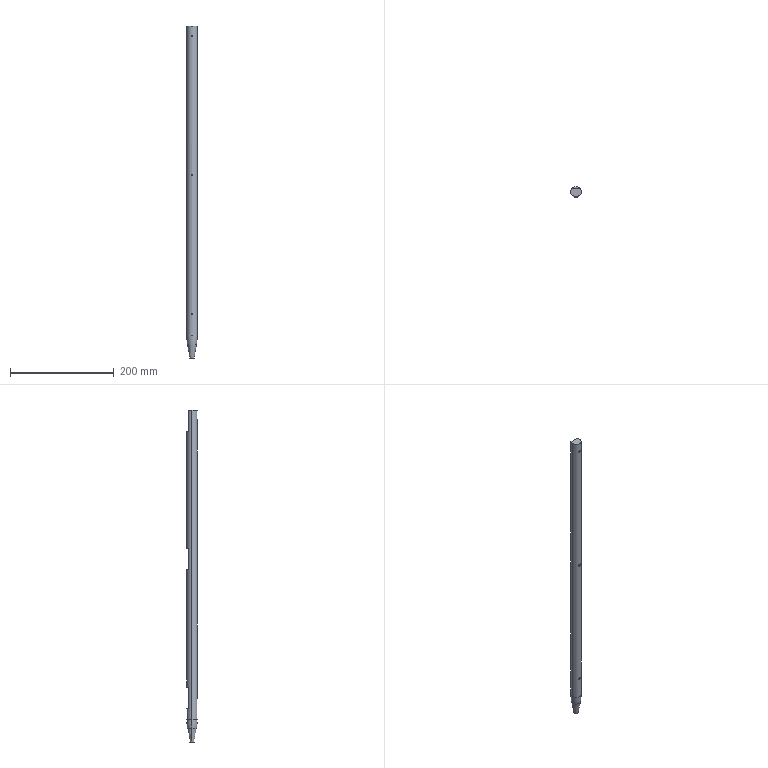Part | STEP file | X77-09002 | 1 solid | 28 faces | box 20 x 20 x 640 mm | volume 189382 mm3 | plane 10 | cylinder 8 | cone 8 | torus 2 | commonest cylinder face diameters 5 x6 20 x2
STEP:
#1=CARTESIAN_POINT('',(-186.5,-272.175,617.5));
#2=VERTEX_POINT('',#1);
#3=CARTESIAN_POINT('',(-186.5,-272.175,622.5));
#4=VERTEX_POINT('',#3);
#5=CARTESIAN_POINT('',(-186.5,-272.175,620.));
#6=DIRECTION('',(0.,1.,0.));
#7=DIRECTION('',(0.,0.,1.));
#8=AXIS2_PLACEMENT_3D('',#5,#6,#7);
#9=CIRCLE('',#8,2.5);
#10=EDGE_CURVE('',#2,#4,#9,.T.);
#11=ORIENTED_EDGE('',*,*,#10,.F.);
#12=CARTESIAN_POINT('',(-186.5,-257.175,617.5));
#13=VERTEX_POINT('',#12);
#14=CARTESIAN_POINT('',(-186.5,-257.175,617.5));
#15=DIRECTION('',(0.,1.,0.));
#16=VECTOR('',#15,1000.);
#17=LINE('',#14,#16);
#18=EDGE_CURVE('',#2,#13,#17,.T.);
#19=ORIENTED_EDGE('',*,*,#18,.T.);
#20=CARTESIAN_POINT('',(-186.5,-257.175,622.5));
#21=VERTEX_POINT('',#20);
#22=CARTESIAN_POINT('',(-186.5,-257.175,620.));
#23=DIRECTION('',(0.,1.,0.));
#24=DIRECTION('',(0.,0.,1.));
#25=AXIS2_PLACEMENT_3D('',#22,#23,#24);
#26=CIRCLE('',#25,2.5);
#27=EDGE_CURVE('',#13,#21,#26,.T.);
#28=ORIENTED_EDGE('',*,*,#27,.T.);
#29=CARTESIAN_POINT('',(-186.5,-257.175,622.5));
#30=DIRECTION('',(0.,1.,0.));
#31=VECTOR('',#30,1000.);
#32=LINE('',#29,#31);
#33=EDGE_CURVE('',#4,#21,#32,.T.);
#34=ORIENTED_EDGE('',*,*,#33,.F.);
#35=EDGE_LOOP('',(#11,#19,#28,#34));
#36=FACE_OUTER_BOUND('',#35,.T.);
#37=CARTESIAN_POINT('',(-186.5,-257.175,620.));
#38=DIRECTION('',(0.,1.,0.));
#39=DIRECTION('',(0.,0.,1.));
#40=AXIS2_PLACEMENT_3D('',#37,#38,#39);
#41=CYLINDRICAL_SURFACE('',#40,2.5);
#42=ADVANCED_FACE('',(#36),#41,.F.);
#43=CARTESIAN_POINT('',(-186.5,-273.175,619.164));
#44=VERTEX_POINT('',#43);
#45=CARTESIAN_POINT('',(-186.5,-273.175,620.836));
#46=VERTEX_POINT('',#45);
#47=CARTESIAN_POINT('',(-186.5,-273.175,619.164));
#48=CARTESIAN_POINT('',(-186.613,-273.175,619.164));
#49=CARTESIAN_POINT('',(-186.728,-273.173,619.184));
#50=CARTESIAN_POINT('',(-186.943,-273.166,619.264));
#51=CARTESIAN_POINT('',(-187.041,-273.161,619.322));
#52=CARTESIAN_POINT('',(-187.212,-273.15,619.475));
#53=CARTESIAN_POINT('',(-187.281,-273.145,619.566));
#54=CARTESIAN_POINT('',(-187.378,-273.137,619.773));
#55=CARTESIAN_POINT('',(-187.404,-273.134,619.886));
#56=CARTESIAN_POINT('',(-187.404,-273.134,620.113));
#57=CARTESIAN_POINT('',(-187.378,-273.137,620.227));
#58=CARTESIAN_POINT('',(-187.282,-273.145,620.433));
#59=CARTESIAN_POINT('',(-187.212,-273.15,620.526));
#60=CARTESIAN_POINT('',(-186.955,-273.166,620.754));
#61=CARTESIAN_POINT('',(-186.728,-273.175,620.836));
#62=CARTESIAN_POINT('',(-186.5,-273.175,620.836));
#63=B_SPLINE_CURVE_WITH_KNOTS('',3,(#47,#48,#49,#50,#51,#52,#53,#54,#55,#56,#57,#58,#59,#60,#61,#62),.UNSPECIFIED.,.F.,.F.,(4,2,2,2,2,2,2,4),(0.00507,0.005409,0.005749,0.006088,0.006428,0.006768,0.007107,0.007786),.UNSPECIFIED.);
#64=EDGE_CURVE('',#44,#46,#63,.T.);
#65=ORIENTED_EDGE('',*,*,#64,.F.);
#66=CARTESIAN_POINT('',(-186.5,-272.175,617.5));
#67=DIRECTION('',(0.,0.515,-0.8572));
#68=VECTOR('',#67,1000.);
#69=LINE('',#66,#68);
#70=EDGE_CURVE('',#44,#2,#69,.T.);
#71=ORIENTED_EDGE('',*,*,#70,.T.);
#72=ORIENTED_EDGE('',*,*,#10,.T.);
#73=CARTESIAN_POINT('',(-186.5,-272.175,622.5));
#74=DIRECTION('',(0.,0.515,0.8572));
#75=VECTOR('',#74,1000.);
#76=LINE('',#73,#75);
#77=EDGE_CURVE('',#46,#4,#76,.T.);
#78=ORIENTED_EDGE('',*,*,#77,.F.);
#79=EDGE_LOOP('',(#65,#71,#72,#78));
#80=FACE_OUTER_BOUND('',#79,.T.);
#81=CARTESIAN_POINT('',(-186.5,-272.175,620.));
#82=DIRECTION('',(0.,1.,0.));
#83=DIRECTION('',(0.,0.,1.));
#84=AXIS2_PLACEMENT_3D('',#81,#82,#83);
#85=CONICAL_SURFACE('',#84,2.5,1.03);
#86=ADVANCED_FACE('',(#80),#85,.F.);
#87=CARTESIAN_POINT('',(-186.5,-272.175,350.));
#88=VERTEX_POINT('',#87);
#89=CARTESIAN_POINT('',(-186.5,-272.175,355.));
#90=VERTEX_POINT('',#89);
#91=CARTESIAN_POINT('',(-186.5,-272.175,352.5));
#92=DIRECTION('',(0.,1.,0.));
#93=DIRECTION('',(0.,0.,1.));
#94=AXIS2_PLACEMENT_3D('',#91,#92,#93);
#95=CIRCLE('',#94,2.5);
#96=EDGE_CURVE('',#88,#90,#95,.T.);
#97=ORIENTED_EDGE('',*,*,#96,.F.);
#98=CARTESIAN_POINT('',(-186.5,-257.175,350.));
#99=VERTEX_POINT('',#98);
#100=CARTESIAN_POINT('',(-186.5,-257.175,350.));
#101=DIRECTION('',(0.,1.,0.));
#102=VECTOR('',#101,1000.);
#103=LINE('',#100,#102);
#104=EDGE_CURVE('',#88,#99,#103,.T.);
#105=ORIENTED_EDGE('',*,*,#104,.T.);
#106=CARTESIAN_POINT('',(-186.5,-257.175,355.));
#107=VERTEX_POINT('',#106);
#108=CARTESIAN_POINT('',(-186.5,-257.175,352.5));
#109=DIRECTION('',(0.,-1.,0.));
#110=DIRECTION('',(0.,0.,1.));
#111=AXIS2_PLACEMENT_3D('',#108,#109,#110);
#112=CIRCLE('',#111,2.5);
#113=EDGE_CURVE('',#107,#99,#112,.T.);
#114=ORIENTED_EDGE('',*,*,#113,.F.);
#115=CARTESIAN_POINT('',(-186.5,-257.175,355.));
#116=DIRECTION('',(0.,1.,0.));
#117=VECTOR('',#116,1000.);
#118=LINE('',#115,#117);
#119=EDGE_CURVE('',#90,#107,#118,.T.);
#120=ORIENTED_EDGE('',*,*,#119,.F.);
#121=EDGE_LOOP('',(#97,#105,#114,#120));
#122=FACE_OUTER_BOUND('',#121,.T.);
#123=CARTESIAN_POINT('',(-186.5,-257.175,352.5));
#124=DIRECTION('',(0.,1.,0.));
#125=DIRECTION('',(0.,0.,1.));
#126=AXIS2_PLACEMENT_3D('',#123,#124,#125);
#127=CYLINDRICAL_SURFACE('',#126,2.5);
#128=ADVANCED_FACE('',(#122),#127,.F.);
#129=CARTESIAN_POINT('',(-186.5,-273.175,351.664));
#130=VERTEX_POINT('',#129);
#131=CARTESIAN_POINT('',(-186.5,-273.175,353.336));
#132=VERTEX_POINT('',#131);
#133=CARTESIAN_POINT('',(-186.5,-273.175,351.664));
#134=CARTESIAN_POINT('',(-186.729,-273.175,351.664));
#135=CARTESIAN_POINT('',(-186.954,-273.166,351.745));
#136=CARTESIAN_POINT('',(-187.211,-273.15,351.974));
#137=CARTESIAN_POINT('',(-187.281,-273.145,352.065));
#138=CARTESIAN_POINT('',(-187.378,-273.137,352.272));
#139=CARTESIAN_POINT('',(-187.404,-273.134,352.386));
#140=CARTESIAN_POINT('',(-187.404,-273.134,352.614));
#141=CARTESIAN_POINT('',(-187.378,-273.137,352.727));
#142=CARTESIAN_POINT('',(-187.281,-273.145,352.935));
#143=CARTESIAN_POINT('',(-187.21,-273.15,353.027));
#144=CARTESIAN_POINT('',(-186.956,-273.166,353.253));
#145=CARTESIAN_POINT('',(-186.727,-273.175,353.336));
#146=CARTESIAN_POINT('',(-186.5,-273.175,353.336));
#147=B_SPLINE_CURVE_WITH_KNOTS('',3,(#133,#134,#135,#136,#137,#138,#139,#140,#141,#142,#143,#144,#145,#146),.UNSPECIFIED.,.F.,.F.,(4,2,2,2,2,2,4),(0.004257,0.004938,0.005279,0.005619,0.00596,0.006301,0.006982),.UNSPECIFIED.);
#148=EDGE_CURVE('',#130,#132,#147,.T.);
#149=ORIENTED_EDGE('',*,*,#148,.F.);
#150=CARTESIAN_POINT('',(-186.5,-272.175,350.));
#151=DIRECTION('',(0.,0.515,-0.8572));
#152=VECTOR('',#151,1000.);
#153=LINE('',#150,#152);
#154=EDGE_CURVE('',#130,#88,#153,.T.);
#155=ORIENTED_EDGE('',*,*,#154,.T.);
#156=ORIENTED_EDGE('',*,*,#96,.T.);
#157=CARTESIAN_POINT('',(-186.5,-272.175,355.));
#158=DIRECTION('',(0.,0.515,0.8572));
#159=VECTOR('',#158,1000.);
#160=LINE('',#157,#159);
#161=EDGE_CURVE('',#132,#90,#160,.T.);
#162=ORIENTED_EDGE('',*,*,#161,.F.);
#163=EDGE_LOOP('',(#149,#155,#156,#162));
#164=FACE_OUTER_BOUND('',#163,.T.);
#165=CARTESIAN_POINT('',(-186.5,-272.175,352.5));
#166=DIRECTION('',(0.,1.,0.));
#167=DIRECTION('',(0.,0.,1.));
#168=AXIS2_PLACEMENT_3D('',#165,#166,#167);
#169=CONICAL_SURFACE('',#168,2.5,1.03);
#170=ADVANCED_FACE('',(#164),#169,.F.);
#171=CARTESIAN_POINT('',(-186.5,-272.175,82.5));
#172=VERTEX_POINT('',#171);
#173=CARTESIAN_POINT('',(-186.5,-272.175,87.5));
#174=VERTEX_POINT('',#173);
#175=CARTESIAN_POINT('',(-186.5,-272.175,85.));
#176=DIRECTION('',(0.,1.,0.));
#177=DIRECTION('',(0.,0.,1.));
#178=AXIS2_PLACEMENT_3D('',#175,#176,#177);
#179=CIRCLE('',#178,2.5);
#180=EDGE_CURVE('',#172,#174,#179,.T.);
#181=ORIENTED_EDGE('',*,*,#180,.F.);
#182=CARTESIAN_POINT('',(-186.5,-257.175,82.5));
#183=VERTEX_POINT('',#182);
#184=CARTESIAN_POINT('',(-186.5,-257.175,82.5));
#185=DIRECTION('',(0.,1.,0.));
#186=VECTOR('',#185,1000.);
#187=LINE('',#184,#186);
#188=EDGE_CURVE('',#172,#183,#187,.T.);
#189=ORIENTED_EDGE('',*,*,#188,.T.);
#190=CARTESIAN_POINT('',(-186.5,-257.175,87.5));
#191=VERTEX_POINT('',#190);
#192=CARTESIAN_POINT('',(-186.5,-257.175,85.));
#193=DIRECTION('',(0.,-1.,0.));
#194=DIRECTION('',(0.,0.,1.));
#195=AXIS2_PLACEMENT_3D('',#192,#193,#194);
#196=CIRCLE('',#195,2.5);
#197=EDGE_CURVE('',#191,#183,#196,.T.);
#198=ORIENTED_EDGE('',*,*,#197,.F.);
#199=CARTESIAN_POINT('',(-186.5,-257.175,87.5));
#200=DIRECTION('',(0.,1.,0.));
#201=VECTOR('',#200,1000.);
#202=LINE('',#199,#201);
#203=EDGE_CURVE('',#174,#191,#202,.T.);
#204=ORIENTED_EDGE('',*,*,#203,.F.);
#205=EDGE_LOOP('',(#181,#189,#198,#204));
#206=FACE_OUTER_BOUND('',#205,.T.);
#207=CARTESIAN_POINT('',(-186.5,-257.175,85.));
#208=DIRECTION('',(0.,1.,0.));
#209=DIRECTION('',(0.,0.,1.));
#210=AXIS2_PLACEMENT_3D('',#207,#208,#209);
#211=CYLINDRICAL_SURFACE('',#210,2.5);
#212=ADVANCED_FACE('',(#206),#211,.F.);
#213=CARTESIAN_POINT('',(-186.5,-273.175,84.164));
#214=VERTEX_POINT('',#213);
#215=CARTESIAN_POINT('',(-186.5,-273.175,85.836));
#216=VERTEX_POINT('',#215);
#217=CARTESIAN_POINT('',(-186.5,-273.175,84.164));
#218=CARTESIAN_POINT('',(-186.729,-273.175,84.164));
#219=CARTESIAN_POINT('',(-186.954,-273.166,84.245));
#220=CARTESIAN_POINT('',(-187.211,-273.15,84.474));
#221=CARTESIAN_POINT('',(-187.281,-273.145,84.565));
#222=CARTESIAN_POINT('',(-187.378,-273.137,84.772));
#223=CARTESIAN_POINT('',(-187.404,-273.134,84.886));
#224=CARTESIAN_POINT('',(-187.404,-273.134,85.114));
#225=CARTESIAN_POINT('',(-187.378,-273.137,85.227));
#226=CARTESIAN_POINT('',(-187.281,-273.145,85.435));
#227=CARTESIAN_POINT('',(-187.21,-273.15,85.527));
#228=CARTESIAN_POINT('',(-186.956,-273.166,85.753));
#229=CARTESIAN_POINT('',(-186.727,-273.175,85.836));
#230=CARTESIAN_POINT('',(-186.5,-273.175,85.836));
#231=B_SPLINE_CURVE_WITH_KNOTS('',3,(#217,#218,#219,#220,#221,#222,#223,#224,#225,#226,#227,#228,#229,#230),.UNSPECIFIED.,.F.,.F.,(4,2,2,2,2,2,4),(0.004257,0.004938,0.005279,0.005619,0.00596,0.006301,0.006982),.UNSPECIFIED.);
#232=EDGE_CURVE('',#214,#216,#231,.T.);
#233=ORIENTED_EDGE('',*,*,#232,.F.);
#234=CARTESIAN_POINT('',(-186.5,-272.175,82.5));
#235=DIRECTION('',(0.,0.515,-0.8572));
#236=VECTOR('',#235,1000.);
#237=LINE('',#234,#236);
#238=EDGE_CURVE('',#214,#172,#237,.T.);
#239=ORIENTED_EDGE('',*,*,#238,.T.);
#240=ORIENTED_EDGE('',*,*,#180,.T.);
#241=CARTESIAN_POINT('',(-186.5,-272.175,87.5));
#242=DIRECTION('',(0.,0.515,0.8572));
#243=VECTOR('',#242,1000.);
#244=LINE('',#241,#243);
#245=EDGE_CURVE('',#216,#174,#244,.T.);
#246=ORIENTED_EDGE('',*,*,#245,.F.);
#247=EDGE_LOOP('',(#233,#239,#240,#246));
#248=FACE_OUTER_BOUND('',#247,.T.);
#249=CARTESIAN_POINT('',(-186.5,-272.175,85.));
#250=DIRECTION('',(0.,1.,0.));
#251=DIRECTION('',(0.,0.,1.));
#252=AXIS2_PLACEMENT_3D('',#249,#250,#251);
#253=CONICAL_SURFACE('',#252,2.5,1.03);
#254=ADVANCED_FACE('',(#248),#253,.F.);
#255=CARTESIAN_POINT('',(-176.5,-263.175,42.777));
#256=VERTEX_POINT('',#255);
#257=CARTESIAN_POINT('',(-196.5,-263.175,42.777));
#258=VERTEX_POINT('',#257);
#259=CARTESIAN_POINT('',(-186.5,-263.175,42.777));
#260=DIRECTION('',(0.,0.,1.));
#261=DIRECTION('',(-1.,0.,0.));
#262=AXIS2_PLACEMENT_3D('',#259,#260,#261);
#263=CIRCLE('',#262,10.);
#264=EDGE_CURVE('',#256,#258,#263,.T.);
#265=ORIENTED_EDGE('',*,*,#264,.F.);
#266=CARTESIAN_POINT('',(-178.019,-263.175,25.412));
#267=VERTEX_POINT('',#266);
#268=CARTESIAN_POINT('',(-276.5,-263.175,42.777));
#269=DIRECTION('',(0.,1.,0.));
#270=DIRECTION('',(-1.,0.,0.));
#271=AXIS2_PLACEMENT_3D('',#268,#269,#270);
#272=CIRCLE('',#271,100.);
#273=EDGE_CURVE('',#256,#267,#272,.T.);
#274=ORIENTED_EDGE('',*,*,#273,.T.);
#275=CARTESIAN_POINT('',(-194.981,-263.175,25.412));
#276=VERTEX_POINT('',#275);
#277=CARTESIAN_POINT('',(-186.5,-263.175,25.412));
#278=DIRECTION('',(0.,0.,-1.));
#279=DIRECTION('',(1.,0.,0.));
#280=AXIS2_PLACEMENT_3D('',#277,#278,#279);
#281=CIRCLE('',#280,8.481);
#282=EDGE_CURVE('',#276,#267,#281,.T.);
#283=ORIENTED_EDGE('',*,*,#282,.F.);
#284=CARTESIAN_POINT('',(-96.5,-263.175,42.777));
#285=DIRECTION('',(0.,-1.,0.));
#286=DIRECTION('',(0.,0.,-1.));
#287=AXIS2_PLACEMENT_3D('',#284,#285,#286);
#288=CIRCLE('',#287,100.);
#289=EDGE_CURVE('',#258,#276,#288,.T.);
#290=ORIENTED_EDGE('',*,*,#289,.F.);
#291=EDGE_LOOP('',(#265,#274,#283,#290));
#292=FACE_OUTER_BOUND('',#291,.T.);
#293=CARTESIAN_POINT('',(-186.5,-263.175,42.777));
#294=DIRECTION('',(0.,0.,-1.));
#295=DIRECTION('',(-1.,0.,0.));
#296=AXIS2_PLACEMENT_3D('',#293,#294,#295);
#297=TOROIDAL_SURFACE('',#296,-90.,100.);
#298=ADVANCED_FACE('',(#292),#297,.T.);
#299=CARTESIAN_POINT('',(-190.5,-263.175,0.));
#300=VERTEX_POINT('',#299);
#301=CARTESIAN_POINT('',(-182.5,-263.175,0.));
#302=VERTEX_POINT('',#301);
#303=CARTESIAN_POINT('',(-186.5,-263.175,0.));
#304=DIRECTION('',(0.,0.,-1.));
#305=DIRECTION('',(1.,0.,0.));
#306=AXIS2_PLACEMENT_3D('',#303,#304,#305);
#307=CIRCLE('',#306,4.);
#308=EDGE_CURVE('',#300,#302,#307,.T.);
#309=ORIENTED_EDGE('',*,*,#308,.F.);
#310=CARTESIAN_POINT('',(-196.5,-263.175,34.028));
#311=DIRECTION('',(-0.1736,0.,0.9848));
#312=VECTOR('',#311,1000.);
#313=LINE('',#310,#312);
#314=EDGE_CURVE('',#300,#276,#313,.T.);
#315=ORIENTED_EDGE('',*,*,#314,.T.);
#316=ORIENTED_EDGE('',*,*,#282,.T.);
#317=CARTESIAN_POINT('',(-176.5,-263.175,34.028));
#318=DIRECTION('',(0.1736,0.,0.9848));
#319=VECTOR('',#318,1000.);
#320=LINE('',#317,#319);
#321=EDGE_CURVE('',#302,#267,#320,.T.);
#322=ORIENTED_EDGE('',*,*,#321,.F.);
#323=EDGE_LOOP('',(#309,#315,#316,#322));
#324=FACE_OUTER_BOUND('',#323,.T.);
#325=CARTESIAN_POINT('',(-186.5,-263.175,34.028));
#326=DIRECTION('',(0.,0.,1.));
#327=DIRECTION('',(1.,0.,0.));
#328=AXIS2_PLACEMENT_3D('',#325,#326,#327);
#329=CONICAL_SURFACE('',#328,10.,0.1745);
#330=ADVANCED_FACE('',(#324),#329,.T.);
#331=CARTESIAN_POINT('',(-178.5,-257.175,106.));
#332=VERTEX_POINT('',#331);
#333=CARTESIAN_POINT('',(-178.5,-257.175,65.));
#334=VERTEX_POINT('',#333);
#335=CARTESIAN_POINT('',(-178.5,-257.175,640.));
#336=DIRECTION('',(0.,0.,-1.));
#337=VECTOR('',#336,1000.);
#338=LINE('',#335,#337);
#339=EDGE_CURVE('',#332,#334,#338,.T.);
#340=ORIENTED_EDGE('',*,*,#339,.F.);
#341=CARTESIAN_POINT('',(-194.5,-257.175,106.));
#342=VERTEX_POINT('',#341);
#343=CARTESIAN_POINT('',(-186.5,-263.175,106.));
#344=DIRECTION('',(0.,0.,-1.));
#345=DIRECTION('',(-1.,0.,0.));
#346=AXIS2_PLACEMENT_3D('',#343,#344,#345);
#347=CIRCLE('',#346,10.);
#348=EDGE_CURVE('',#342,#332,#347,.T.);
#349=ORIENTED_EDGE('',*,*,#348,.F.);
#350=CARTESIAN_POINT('',(-194.5,-257.175,65.));
#351=VERTEX_POINT('',#350);
#352=CARTESIAN_POINT('',(-194.5,-257.175,640.));
#353=DIRECTION('',(0.,0.,1.));
#354=VECTOR('',#353,1000.);
#355=LINE('',#352,#354);
#356=EDGE_CURVE('',#351,#342,#355,.T.);
#357=ORIENTED_EDGE('',*,*,#356,.F.);
#358=CARTESIAN_POINT('',(-186.5,-263.175,65.));
#359=DIRECTION('',(0.,0.,1.));
#360=DIRECTION('',(1.,0.,0.));
#361=AXIS2_PLACEMENT_3D('',#358,#359,#360);
#362=CIRCLE('',#361,10.);
#363=EDGE_CURVE('',#334,#351,#362,.T.);
#364=ORIENTED_EDGE('',*,*,#363,.F.);
#365=EDGE_LOOP('',(#340,#349,#357,#364));
#366=FACE_BOUND('',#365,.T.);
#367=CARTESIAN_POINT('',(-178.5,-257.175,373.));
#368=VERTEX_POINT('',#367);
#369=CARTESIAN_POINT('',(-178.5,-257.175,332.));
#370=VERTEX_POINT('',#369);
#371=CARTESIAN_POINT('',(-178.5,-257.175,640.));
#372=DIRECTION('',(0.,0.,-1.));
#373=VECTOR('',#372,1000.);
#374=LINE('',#371,#373);
#375=EDGE_CURVE('',#368,#370,#374,.T.);
#376=ORIENTED_EDGE('',*,*,#375,.F.);
#377=CARTESIAN_POINT('',(-194.5,-257.175,373.));
#378=VERTEX_POINT('',#377);
#379=CARTESIAN_POINT('',(-186.5,-263.175,373.));
#380=DIRECTION('',(0.,0.,-1.));
#381=DIRECTION('',(-1.,0.,0.));
#382=AXIS2_PLACEMENT_3D('',#379,#380,#381);
#383=CIRCLE('',#382,10.);
#384=EDGE_CURVE('',#378,#368,#383,.T.);
#385=ORIENTED_EDGE('',*,*,#384,.F.);
#386=CARTESIAN_POINT('',(-194.5,-257.175,332.));
#387=VERTEX_POINT('',#386);
#388=CARTESIAN_POINT('',(-194.5,-257.175,640.));
#389=DIRECTION('',(0.,0.,1.));
#390=VECTOR('',#389,1000.);
#391=LINE('',#388,#390);
#392=EDGE_CURVE('',#387,#378,#391,.T.);
#393=ORIENTED_EDGE('',*,*,#392,.F.);
#394=CARTESIAN_POINT('',(-186.5,-263.175,332.));
#395=DIRECTION('',(0.,0.,1.));
#396=DIRECTION('',(1.,0.,0.));
#397=AXIS2_PLACEMENT_3D('',#394,#395,#396);
#398=CIRCLE('',#397,10.);
#399=EDGE_CURVE('',#370,#387,#398,.T.);
#400=ORIENTED_EDGE('',*,*,#399,.F.);
#401=EDGE_LOOP('',(#376,#385,#393,#400));
#402=FACE_BOUND('',#401,.T.);
#403=CARTESIAN_POINT('',(-176.5,-263.175,640.));
#404=VERTEX_POINT('',#403);
#405=CARTESIAN_POINT('',(-178.5,-257.175,640.));
#406=VERTEX_POINT('',#405);
#407=CARTESIAN_POINT('',(-186.5,-263.175,640.));
#408=DIRECTION('',(0.,0.,1.));
#409=DIRECTION('',(1.,0.,0.));
#410=AXIS2_PLACEMENT_3D('',#407,#408,#409);
#411=CIRCLE('',#410,10.);
#412=EDGE_CURVE('',#404,#406,#411,.T.);
#413=ORIENTED_EDGE('',*,*,#412,.F.);
#414=CARTESIAN_POINT('',(-176.5,-263.175,640.));
#415=DIRECTION('',(0.,0.,-1.));
#416=VECTOR('',#415,1000.);
#417=LINE('',#414,#416);
#418=EDGE_CURVE('',#404,#256,#417,.T.);
#419=ORIENTED_EDGE('',*,*,#418,.T.);
#420=ORIENTED_EDGE('',*,*,#264,.T.);
#421=CARTESIAN_POINT('',(-196.5,-263.175,640.));
#422=VERTEX_POINT('',#421);
#423=CARTESIAN_POINT('',(-196.5,-263.175,640.));
#424=DIRECTION('',(0.,0.,-1.));
#425=VECTOR('',#424,1000.);
#426=LINE('',#423,#425);
#427=EDGE_CURVE('',#422,#258,#426,.T.);
#428=ORIENTED_EDGE('',*,*,#427,.F.);
#429=CARTESIAN_POINT('',(-194.5,-257.175,640.));
#430=VERTEX_POINT('',#429);
#431=CARTESIAN_POINT('',(-186.5,-263.175,640.));
#432=DIRECTION('',(0.,0.,1.));
#433=DIRECTION('',(1.,0.,0.));
#434=AXIS2_PLACEMENT_3D('',#431,#432,#433);
#435=CIRCLE('',#434,10.);
#436=EDGE_CURVE('',#430,#422,#435,.T.);
#437=ORIENTED_EDGE('',*,*,#436,.F.);
#438=CARTESIAN_POINT('',(-194.5,-257.175,599.));
#439=VERTEX_POINT('',#438);
#440=CARTESIAN_POINT('',(-194.5,-257.175,640.));
#441=DIRECTION('',(0.,0.,-1.));
#442=VECTOR('',#441,1000.);
#443=LINE('',#440,#442);
#444=EDGE_CURVE('',#430,#439,#443,.T.);
#445=ORIENTED_EDGE('',*,*,#444,.T.);
#446=CARTESIAN_POINT('',(-178.5,-257.175,599.));
#447=VERTEX_POINT('',#446);
#448=CARTESIAN_POINT('',(-186.5,-263.175,599.));
#449=DIRECTION('',(0.,0.,-1.));
#450=DIRECTION('',(-1.,0.,0.));
#451=AXIS2_PLACEMENT_3D('',#448,#449,#450);
#452=CIRCLE('',#451,10.);
#453=EDGE_CURVE('',#439,#447,#452,.T.);
#454=ORIENTED_EDGE('',*,*,#453,.T.);
#455=CARTESIAN_POINT('',(-178.5,-257.175,640.));
#456=DIRECTION('',(0.,0.,1.));
#457=VECTOR('',#456,1000.);
#458=LINE('',#455,#457);
#459=EDGE_CURVE('',#447,#406,#458,.T.);
#460=ORIENTED_EDGE('',*,*,#459,.T.);
#461=EDGE_LOOP('',(#413,#419,#420,#428,#437,#445,#454,#460));
#462=FACE_OUTER_BOUND('',#461,.T.);
#463=CARTESIAN_POINT('',(-186.5,-263.175,640.));
#464=DIRECTION('',(0.,0.,-1.));
#465=DIRECTION('',(-1.,0.,0.));
#466=AXIS2_PLACEMENT_3D('',#463,#464,#465);
#467=CYLINDRICAL_SURFACE('',#466,10.);
#468=ADVANCED_FACE('',(#366,#402,#462),#467,.T.);
#469=ORIENTED_EDGE('',*,*,#418,.F.);
#470=CARTESIAN_POINT('',(-186.5,-263.175,640.));
#471=DIRECTION('',(0.,0.,1.));
#472=DIRECTION('',(1.,0.,0.));
#473=AXIS2_PLACEMENT_3D('',#470,#471,#472);
#474=CIRCLE('',#473,10.);
#475=EDGE_CURVE('',#422,#404,#474,.T.);
#476=ORIENTED_EDGE('',*,*,#475,.F.);
#477=ORIENTED_EDGE('',*,*,#427,.T.);
#478=CARTESIAN_POINT('',(-186.5,-263.175,42.777));
#479=DIRECTION('',(0.,0.,1.));
#480=DIRECTION('',(-1.,0.,0.));
#481=AXIS2_PLACEMENT_3D('',#478,#479,#480);
#482=CIRCLE('',#481,10.);
#483=EDGE_CURVE('',#258,#256,#482,.T.);
#484=ORIENTED_EDGE('',*,*,#483,.T.);
#485=EDGE_LOOP('',(#469,#476,#477,#484));
#486=FACE_OUTER_BOUND('',#485,.T.);
#487=CARTESIAN_POINT('',(-186.5,-273.175,620.836));
#488=CARTESIAN_POINT('',(-186.386,-273.175,620.836));
#489=CARTESIAN_POINT('',(-186.272,-273.173,620.815));
#490=CARTESIAN_POINT('',(-186.059,-273.166,620.737));
#491=CARTESIAN_POINT('',(-185.959,-273.161,620.678));
#492=CARTESIAN_POINT('',(-185.79,-273.15,620.527));
#493=CARTESIAN_POINT('',(-185.719,-273.145,620.434));
#494=CARTESIAN_POINT('',(-185.623,-273.137,620.23));
#495=CARTESIAN_POINT('',(-185.596,-273.134,620.115));
#496=CARTESIAN_POINT('',(-185.596,-273.134,619.888));
#497=CARTESIAN_POINT('',(-185.621,-273.137,619.774));
#498=CARTESIAN_POINT('',(-185.718,-273.145,619.566));
#499=CARTESIAN_POINT('',(-185.789,-273.15,619.474));
#500=CARTESIAN_POINT('',(-186.044,-273.166,619.247));
#501=CARTESIAN_POINT('',(-186.273,-273.175,619.164));
#502=CARTESIAN_POINT('',(-186.5,-273.175,619.164));
#503=B_SPLINE_CURVE_WITH_KNOTS('',3,(#487,#488,#489,#490,#491,#492,#493,#494,#495,#496,#497,#498,#499,#500,#501,#502),.UNSPECIFIED.,.F.,.F.,(4,2,2,2,2,2,2,4),(0.002352,0.002692,0.003032,0.003371,0.003711,0.004051,0.00439,0.00507),.UNSPECIFIED.);
#504=EDGE_CURVE('',#46,#44,#503,.T.);
#505=ORIENTED_EDGE('',*,*,#504,.T.);
#506=ORIENTED_EDGE('',*,*,#64,.T.);
#507=EDGE_LOOP('',(#505,#506));
#508=FACE_BOUND('',#507,.T.);
#509=CARTESIAN_POINT('',(-186.5,-273.175,353.336));
#510=CARTESIAN_POINT('',(-186.273,-273.175,353.336));
#511=CARTESIAN_POINT('',(-186.044,-273.166,353.253));
#512=CARTESIAN_POINT('',(-185.79,-273.15,353.027));
#513=CARTESIAN_POINT('',(-185.72,-273.145,352.935));
#514=CARTESIAN_POINT('',(-185.623,-273.137,352.729));
#515=CARTESIAN_POINT('',(-185.596,-273.134,352.616));
#516=CARTESIAN_POINT('',(-185.596,-273.134,352.386));
#517=CARTESIAN_POINT('',(-185.622,-273.137,352.273));
#518=CARTESIAN_POINT('',(-185.718,-273.145,352.067));
#519=CARTESIAN_POINT('',(-185.789,-273.15,351.974));
#520=CARTESIAN_POINT('',(-185.959,-273.161,351.823));
#521=CARTESIAN_POINT('',(-186.058,-273.166,351.764));
#522=CARTESIAN_POINT('',(-186.272,-273.173,351.684));
#523=CARTESIAN_POINT('',(-186.386,-273.175,351.664));
#524=CARTESIAN_POINT('',(-186.5,-273.175,351.664));
#525=B_SPLINE_CURVE_WITH_KNOTS('',3,(#509,#510,#511,#512,#513,#514,#515,#516,#517,#518,#519,#520,#521,#522,#523,#524),.UNSPECIFIED.,.F.,.F.,(4,2,2,2,2,2,2,4),(0.00153,0.002212,0.002553,0.002893,0.003234,0.003575,0.003916,0.004257),.UNSPECIFIED.);
#526=EDGE_CURVE('',#132,#130,#525,.T.);
#527=ORIENTED_EDGE('',*,*,#526,.T.);
#528=ORIENTED_EDGE('',*,*,#148,.T.);
#529=EDGE_LOOP('',(#527,#528));
#530=FACE_BOUND('',#529,.T.);
#531=CARTESIAN_POINT('',(-186.5,-273.175,85.836));
#532=CARTESIAN_POINT('',(-186.273,-273.175,85.836));
#533=CARTESIAN_POINT('',(-186.044,-273.166,85.753));
#534=CARTESIAN_POINT('',(-185.79,-273.15,85.527));
#535=CARTESIAN_POINT('',(-185.72,-273.145,85.435));
#536=CARTESIAN_POINT('',(-185.623,-273.137,85.229));
#537=CARTESIAN_POINT('',(-185.596,-273.134,85.116));
#538=CARTESIAN_POINT('',(-185.596,-273.134,84.886));
#539=CARTESIAN_POINT('',(-185.622,-273.137,84.773));
#540=CARTESIAN_POINT('',(-185.718,-273.145,84.567));
#541=CARTESIAN_POINT('',(-185.789,-273.15,84.474));
#542=CARTESIAN_POINT('',(-185.959,-273.161,84.323));
#543=CARTESIAN_POINT('',(-186.058,-273.166,84.264));
#544=CARTESIAN_POINT('',(-186.272,-273.173,84.184));
#545=CARTESIAN_POINT('',(-186.386,-273.175,84.164));
#546=CARTESIAN_POINT('',(-186.5,-273.175,84.164));
#547=B_SPLINE_CURVE_WITH_KNOTS('',3,(#531,#532,#533,#534,#535,#536,#537,#538,#539,#540,#541,#542,#543,#544,#545,#546),.UNSPECIFIED.,.F.,.F.,(4,2,2,2,2,2,2,4),(0.00153,0.002212,0.002553,0.002893,0.003234,0.003575,0.003916,0.004257),.UNSPECIFIED.);
#548=EDGE_CURVE('',#216,#214,#547,.T.);
#549=ORIENTED_EDGE('',*,*,#548,.T.);
#550=ORIENTED_EDGE('',*,*,#232,.T.);
#551=EDGE_LOOP('',(#549,#550));
#552=FACE_BOUND('',#551,.T.);
#553=CARTESIAN_POINT('',(-186.5,-263.175,640.));
#554=DIRECTION('',(0.,0.,-1.));
#555=DIRECTION('',(-1.,0.,0.));
#556=AXIS2_PLACEMENT_3D('',#553,#554,#555);
#557=CYLINDRICAL_SURFACE('',#556,10.);
#558=ADVANCED_FACE('',(#486,#508,#530,#552),#557,.T.);
#559=CARTESIAN_POINT('',(-186.5,-257.175,640.));
#560=DIRECTION('',(1.,0.,0.));
#561=VECTOR('',#560,1000.);
#562=LINE('',#559,#561);
#563=EDGE_CURVE('',#430,#406,#562,.T.);
#564=ORIENTED_EDGE('',*,*,#563,.F.);
#565=ORIENTED_EDGE('',*,*,#436,.T.);
#566=ORIENTED_EDGE('',*,*,#475,.T.);
#567=ORIENTED_EDGE('',*,*,#412,.T.);
#568=EDGE_LOOP('',(#564,#565,#566,#567));
#569=FACE_OUTER_BOUND('',#568,.T.);
#570=CARTESIAN_POINT('',(-186.5,-263.175,640.));
#571=DIRECTION('',(0.,0.,1.));
#572=DIRECTION('',(1.,0.,0.));
#573=AXIS2_PLACEMENT_3D('',#570,#571,#572);
#574=PLANE('',#573);
#575=ADVANCED_FACE('',(#569),#574,.T.);
#576=CARTESIAN_POINT('',(-186.5,-263.175,0.));
#577=DIRECTION('',(0.,0.,-1.));
#578=DIRECTION('',(1.,0.,0.));
#579=AXIS2_PLACEMENT_3D('',#576,#577,#578);
#580=CIRCLE('',#579,4.);
#581=EDGE_CURVE('',#302,#300,#580,.T.);
#582=ORIENTED_EDGE('',*,*,#581,.T.);
#583=ORIENTED_EDGE('',*,*,#308,.T.);
#584=EDGE_LOOP('',(#582,#583));
#585=FACE_OUTER_BOUND('',#584,.T.);
#586=CARTESIAN_POINT('',(-186.5,-263.175,0.));
#587=DIRECTION('',(0.,0.,1.));
#588=DIRECTION('',(1.,0.,0.));
#589=AXIS2_PLACEMENT_3D('',#586,#587,#588);
#590=PLANE('',#589);
#591=ADVANCED_FACE('',(#585),#590,.F.);
#592=ORIENTED_EDGE('',*,*,#314,.F.);
#593=ORIENTED_EDGE('',*,*,#581,.F.);
#594=ORIENTED_EDGE('',*,*,#321,.T.);
#595=CARTESIAN_POINT('',(-186.5,-263.175,25.412));
#596=DIRECTION('',(0.,0.,-1.));
#597=DIRECTION('',(1.,0.,0.));
#598=AXIS2_PLACEMENT_3D('',#595,#596,#597);
#599=CIRCLE('',#598,8.481);
#600=EDGE_CURVE('',#267,#276,#599,.T.);
#601=ORIENTED_EDGE('',*,*,#600,.T.);
#602=EDGE_LOOP('',(#592,#593,#594,#601));
#603=FACE_OUTER_BOUND('',#602,.T.);
#604=CARTESIAN_POINT('',(-186.5,-263.175,34.028));
#605=DIRECTION('',(0.,0.,1.));
#606=DIRECTION('',(1.,0.,0.));
#607=AXIS2_PLACEMENT_3D('',#604,#605,#606);
#608=CONICAL_SURFACE('',#607,10.,0.1745);
#609=ADVANCED_FACE('',(#603),#608,.T.);
#610=ORIENTED_EDGE('',*,*,#273,.F.);
#611=ORIENTED_EDGE('',*,*,#483,.F.);
#612=ORIENTED_EDGE('',*,*,#289,.T.);
#613=ORIENTED_EDGE('',*,*,#600,.F.);
#614=EDGE_LOOP('',(#610,#611,#612,#613));
#615=FACE_OUTER_BOUND('',#614,.T.);
#616=CARTESIAN_POINT('',(-186.5,-263.175,42.777));
#617=DIRECTION('',(0.,0.,-1.));
#618=DIRECTION('',(-1.,0.,0.));
#619=AXIS2_PLACEMENT_3D('',#616,#617,#618);
#620=TOROIDAL_SURFACE('',#619,-90.,100.);
#621=ADVANCED_FACE('',(#615),#620,.T.);
#622=CARTESIAN_POINT('',(-198.415,-257.175,599.));
#623=DIRECTION('',(1.,0.,0.));
#624=VECTOR('',#623,1000.);
#625=LINE('',#622,#624);
#626=EDGE_CURVE('',#439,#447,#625,.T.);
#627=ORIENTED_EDGE('',*,*,#626,.T.);
#628=ORIENTED_EDGE('',*,*,#453,.F.);
#629=EDGE_LOOP('',(#627,#628));
#630=FACE_OUTER_BOUND('',#629,.T.);
#631=CARTESIAN_POINT('',(-198.415,-251.133,599.));
#632=DIRECTION('',(0.,0.,-1.));
#633=DIRECTION('',(-1.,0.,0.));
#634=AXIS2_PLACEMENT_3D('',#631,#632,#633);
#635=PLANE('',#634);
#636=ADVANCED_FACE('',(#630),#635,.F.);
#637=CARTESIAN_POINT('',(-186.5,-257.175,620.));
#638=DIRECTION('',(0.,1.,0.));
#639=DIRECTION('',(0.,0.,1.));
#640=AXIS2_PLACEMENT_3D('',#637,#638,#639);
#641=CIRCLE('',#640,2.5);
#642=EDGE_CURVE('',#21,#13,#641,.T.);
#643=ORIENTED_EDGE('',*,*,#642,.F.);
#644=ORIENTED_EDGE('',*,*,#27,.F.);
#645=EDGE_LOOP('',(#643,#644));
#646=FACE_BOUND('',#645,.T.);
#647=ORIENTED_EDGE('',*,*,#563,.T.);
#648=ORIENTED_EDGE('',*,*,#459,.F.);
#649=ORIENTED_EDGE('',*,*,#626,.F.);
#650=ORIENTED_EDGE('',*,*,#444,.F.);
#651=EDGE_LOOP('',(#647,#648,#649,#650));
#652=FACE_OUTER_BOUND('',#651,.T.);
#653=CARTESIAN_POINT('',(-198.415,-257.175,599.));
#654=DIRECTION('',(0.,-1.,0.));
#655=DIRECTION('',(0.,0.,-1.));
#656=AXIS2_PLACEMENT_3D('',#653,#654,#655);
#657=PLANE('',#656);
#658=ADVANCED_FACE('',(#646,#652),#657,.F.);
#659=ORIENTED_EDGE('',*,*,#238,.F.);
#660=ORIENTED_EDGE('',*,*,#548,.F.);
#661=ORIENTED_EDGE('',*,*,#245,.T.);
#662=CARTESIAN_POINT('',(-186.5,-272.175,85.));
#663=DIRECTION('',(0.,1.,0.));
#664=DIRECTION('',(0.,0.,1.));
#665=AXIS2_PLACEMENT_3D('',#662,#663,#664);
#666=CIRCLE('',#665,2.5);
#667=EDGE_CURVE('',#174,#172,#666,.T.);
#668=ORIENTED_EDGE('',*,*,#667,.T.);
#669=EDGE_LOOP('',(#659,#660,#661,#668));
#670=FACE_OUTER_BOUND('',#669,.T.);
#671=CARTESIAN_POINT('',(-186.5,-272.175,85.));
#672=DIRECTION('',(0.,1.,0.));
#673=DIRECTION('',(0.,0.,1.));
#674=AXIS2_PLACEMENT_3D('',#671,#672,#673);
#675=CONICAL_SURFACE('',#674,2.5,1.03);
#676=ADVANCED_FACE('',(#670),#675,.F.);
#677=ORIENTED_EDGE('',*,*,#188,.F.);
#678=ORIENTED_EDGE('',*,*,#667,.F.);
#679=ORIENTED_EDGE('',*,*,#203,.T.);
#680=CARTESIAN_POINT('',(-186.5,-257.175,85.));
#681=DIRECTION('',(0.,-1.,0.));
#682=DIRECTION('',(0.,0.,1.));
#683=AXIS2_PLACEMENT_3D('',#680,#681,#682);
#684=CIRCLE('',#683,2.5);
#685=EDGE_CURVE('',#183,#191,#684,.T.);
#686=ORIENTED_EDGE('',*,*,#685,.F.);
#687=EDGE_LOOP('',(#677,#678,#679,#686));
#688=FACE_OUTER_BOUND('',#687,.T.);
#689=CARTESIAN_POINT('',(-186.5,-257.175,85.));
#690=DIRECTION('',(0.,1.,0.));
#691=DIRECTION('',(0.,0.,1.));
#692=AXIS2_PLACEMENT_3D('',#689,#690,#691);
#693=CYLINDRICAL_SURFACE('',#692,2.5);
#694=ADVANCED_FACE('',(#688),#693,.F.);
#695=ORIENTED_EDGE('',*,*,#154,.F.);
#696=ORIENTED_EDGE('',*,*,#526,.F.);
#697=ORIENTED_EDGE('',*,*,#161,.T.);
#698=CARTESIAN_POINT('',(-186.5,-272.175,352.5));
#699=DIRECTION('',(0.,1.,0.));
#700=DIRECTION('',(0.,0.,1.));
#701=AXIS2_PLACEMENT_3D('',#698,#699,#700);
#702=CIRCLE('',#701,2.5);
#703=EDGE_CURVE('',#90,#88,#702,.T.);
#704=ORIENTED_EDGE('',*,*,#703,.T.);
#705=EDGE_LOOP('',(#695,#696,#697,#704));
#706=FACE_OUTER_BOUND('',#705,.T.);
#707=CARTESIAN_POINT('',(-186.5,-272.175,352.5));
#708=DIRECTION('',(0.,1.,0.));
#709=DIRECTION('',(0.,0.,1.));
#710=AXIS2_PLACEMENT_3D('',#707,#708,#709);
#711=CONICAL_SURFACE('',#710,2.5,1.03);
#712=ADVANCED_FACE('',(#706),#711,.F.);
#713=ORIENTED_EDGE('',*,*,#104,.F.);
#714=ORIENTED_EDGE('',*,*,#703,.F.);
#715=ORIENTED_EDGE('',*,*,#119,.T.);
#716=CARTESIAN_POINT('',(-186.5,-257.175,352.5));
#717=DIRECTION('',(0.,-1.,0.));
#718=DIRECTION('',(0.,0.,1.));
#719=AXIS2_PLACEMENT_3D('',#716,#717,#718);
#720=CIRCLE('',#719,2.5);
#721=EDGE_CURVE('',#99,#107,#720,.T.);
#722=ORIENTED_EDGE('',*,*,#721,.F.);
#723=EDGE_LOOP('',(#713,#714,#715,#722));
#724=FACE_OUTER_BOUND('',#723,.T.);
#725=CARTESIAN_POINT('',(-186.5,-257.175,352.5));
#726=DIRECTION('',(0.,1.,0.));
#727=DIRECTION('',(0.,0.,1.));
#728=AXIS2_PLACEMENT_3D('',#725,#726,#727);
#729=CYLINDRICAL_SURFACE('',#728,2.5);
#730=ADVANCED_FACE('',(#724),#729,.F.);
#731=ORIENTED_EDGE('',*,*,#70,.F.);
#732=ORIENTED_EDGE('',*,*,#504,.F.);
#733=ORIENTED_EDGE('',*,*,#77,.T.);
#734=CARTESIAN_POINT('',(-186.5,-272.175,620.));
#735=DIRECTION('',(0.,1.,0.));
#736=DIRECTION('',(0.,0.,1.));
#737=AXIS2_PLACEMENT_3D('',#734,#735,#736);
#738=CIRCLE('',#737,2.5);
#739=EDGE_CURVE('',#4,#2,#738,.T.);
#740=ORIENTED_EDGE('',*,*,#739,.T.);
#741=EDGE_LOOP('',(#731,#732,#733,#740));
#742=FACE_OUTER_BOUND('',#741,.T.);
#743=CARTESIAN_POINT('',(-186.5,-272.175,620.));
#744=DIRECTION('',(0.,1.,0.));
#745=DIRECTION('',(0.,0.,1.));
#746=AXIS2_PLACEMENT_3D('',#743,#744,#745);
#747=CONICAL_SURFACE('',#746,2.5,1.03);
#748=ADVANCED_FACE('',(#742),#747,.F.);
#749=ORIENTED_EDGE('',*,*,#18,.F.);
#750=ORIENTED_EDGE('',*,*,#739,.F.);
#751=ORIENTED_EDGE('',*,*,#33,.T.);
#752=ORIENTED_EDGE('',*,*,#642,.T.);
#753=EDGE_LOOP('',(#749,#750,#751,#752));
#754=FACE_OUTER_BOUND('',#753,.T.);
#755=CARTESIAN_POINT('',(-186.5,-257.175,620.));
#756=DIRECTION('',(0.,1.,0.));
#757=DIRECTION('',(0.,0.,1.));
#758=AXIS2_PLACEMENT_3D('',#755,#756,#757);
#759=CYLINDRICAL_SURFACE('',#758,2.5);
#760=ADVANCED_FACE('',(#754),#759,.F.);
#761=ORIENTED_EDGE('',*,*,#384,.T.);
#762=CARTESIAN_POINT('',(-210.974,-257.175,373.));
#763=DIRECTION('',(1.,0.,0.));
#764=VECTOR('',#763,1000.);
#765=LINE('',#762,#764);
#766=EDGE_CURVE('',#378,#368,#765,.T.);
#767=ORIENTED_EDGE('',*,*,#766,.F.);
#768=EDGE_LOOP('',(#761,#767));
#769=FACE_OUTER_BOUND('',#768,.T.);
#770=CARTESIAN_POINT('',(-210.974,-253.175,373.));
#771=DIRECTION('',(0.,0.,-1.));
#772=DIRECTION('',(-1.,0.,0.));
#773=AXIS2_PLACEMENT_3D('',#770,#771,#772);
#774=PLANE('',#773);
#775=ADVANCED_FACE('',(#769),#774,.T.);
#776=CARTESIAN_POINT('',(-210.974,-257.175,332.));
#777=DIRECTION('',(-1.,0.,0.));
#778=VECTOR('',#777,1000.);
#779=LINE('',#776,#778);
#780=EDGE_CURVE('',#370,#387,#779,.T.);
#781=ORIENTED_EDGE('',*,*,#780,.F.);
#782=ORIENTED_EDGE('',*,*,#399,.T.);
#783=EDGE_LOOP('',(#781,#782));
#784=FACE_OUTER_BOUND('',#783,.T.);
#785=CARTESIAN_POINT('',(-210.974,-253.175,332.));
#786=DIRECTION('',(0.,0.,1.));
#787=DIRECTION('',(1.,0.,0.));
#788=AXIS2_PLACEMENT_3D('',#785,#786,#787);
#789=PLANE('',#788);
#790=ADVANCED_FACE('',(#784),#789,.T.);
#791=ORIENTED_EDGE('',*,*,#113,.T.);
#792=ORIENTED_EDGE('',*,*,#721,.T.);
#793=EDGE_LOOP('',(#791,#792));
#794=FACE_BOUND('',#793,.T.);
#795=ORIENTED_EDGE('',*,*,#375,.T.);
#796=ORIENTED_EDGE('',*,*,#780,.T.);
#797=ORIENTED_EDGE('',*,*,#392,.T.);
#798=ORIENTED_EDGE('',*,*,#766,.T.);
#799=EDGE_LOOP('',(#795,#796,#797,#798));
#800=FACE_OUTER_BOUND('',#799,.T.);
#801=CARTESIAN_POINT('',(-210.974,-257.175,373.));
#802=DIRECTION('',(0.,1.,0.));
#803=DIRECTION('',(0.,0.,1.));
#804=AXIS2_PLACEMENT_3D('',#801,#802,#803);
#805=PLANE('',#804);
#806=ADVANCED_FACE('',(#794,#800),#805,.T.);
#807=ORIENTED_EDGE('',*,*,#348,.T.);
#808=CARTESIAN_POINT('',(-220.621,-257.175,106.));
#809=DIRECTION('',(1.,0.,0.));
#810=VECTOR('',#809,1000.);
#811=LINE('',#808,#810);
#812=EDGE_CURVE('',#342,#332,#811,.T.);
#813=ORIENTED_EDGE('',*,*,#812,.F.);
#814=EDGE_LOOP('',(#807,#813));
#815=FACE_OUTER_BOUND('',#814,.T.);
#816=CARTESIAN_POINT('',(-220.621,-253.175,106.));
#817=DIRECTION('',(0.,0.,-1.));
#818=DIRECTION('',(-1.,0.,0.));
#819=AXIS2_PLACEMENT_3D('',#816,#817,#818);
#820=PLANE('',#819);
#821=ADVANCED_FACE('',(#815),#820,.T.);
#822=CARTESIAN_POINT('',(-220.621,-257.175,65.));
#823=DIRECTION('',(-1.,0.,0.));
#824=VECTOR('',#823,1000.);
#825=LINE('',#822,#824);
#826=EDGE_CURVE('',#334,#351,#825,.T.);
#827=ORIENTED_EDGE('',*,*,#826,.F.);
#828=ORIENTED_EDGE('',*,*,#363,.T.);
#829=EDGE_LOOP('',(#827,#828));
#830=FACE_OUTER_BOUND('',#829,.T.);
#831=CARTESIAN_POINT('',(-220.621,-253.175,65.));
#832=DIRECTION('',(0.,0.,1.));
#833=DIRECTION('',(1.,0.,0.));
#834=AXIS2_PLACEMENT_3D('',#831,#832,#833);
#835=PLANE('',#834);
#836=ADVANCED_FACE('',(#830),#835,.T.);
#837=ORIENTED_EDGE('',*,*,#197,.T.);
#838=ORIENTED_EDGE('',*,*,#685,.T.);
#839=EDGE_LOOP('',(#837,#838));
#840=FACE_BOUND('',#839,.T.);
#841=ORIENTED_EDGE('',*,*,#339,.T.);
#842=ORIENTED_EDGE('',*,*,#826,.T.);
#843=ORIENTED_EDGE('',*,*,#356,.T.);
#844=ORIENTED_EDGE('',*,*,#812,.T.);
#845=EDGE_LOOP('',(#841,#842,#843,#844));
#846=FACE_OUTER_BOUND('',#845,.T.);
#847=CARTESIAN_POINT('',(-220.621,-257.175,106.));
#848=DIRECTION('',(0.,1.,0.));
#849=DIRECTION('',(0.,0.,1.));
#850=AXIS2_PLACEMENT_3D('',#847,#848,#849);
#851=PLANE('',#850);
#852=ADVANCED_FACE('',(#840,#846),#851,.T.);
#853=CLOSED_SHELL('',(#42,#86,#128,#170,#212,#254,#298,#330,#468,#558,#575,#591,#609,#621,#636,#658,#676,#694,#712,#730,#748,#760,#775,#790,#806,#821,#836,#852));
#854=MANIFOLD_SOLID_BREP('',#853);
#855=CARTESIAN_POINT('',(0.,0.,0.));
#856=DIRECTION('',(0.,0.,1.));
#857=DIRECTION('',(1.,0.,0.));
#858=AXIS2_PLACEMENT_3D('',#855,#856,#857);
#859=(LENGTH_UNIT()NAMED_UNIT(*)SI_UNIT(.MILLI.,.METRE.));
#860=UNCERTAINTY_MEASURE_WITH_UNIT(LENGTH_MEASURE(0.00001),#859,'','');
#861=(NAMED_UNIT(*)PLANE_ANGLE_UNIT()SI_UNIT($,.RADIAN.));
#862=(NAMED_UNIT(*)SI_UNIT($,.STERADIAN.)SOLID_ANGLE_UNIT());
#863=(GEOMETRIC_REPRESENTATION_CONTEXT(3)GLOBAL_UNCERTAINTY_ASSIGNED_CONTEXT((#860))GLOBAL_UNIT_ASSIGNED_CONTEXT((#859,#861,#862))REPRESENTATION_CONTEXT('',''));
#864=ADVANCED_BREP_SHAPE_REPRESENTATION('',(#854,#858),#863);